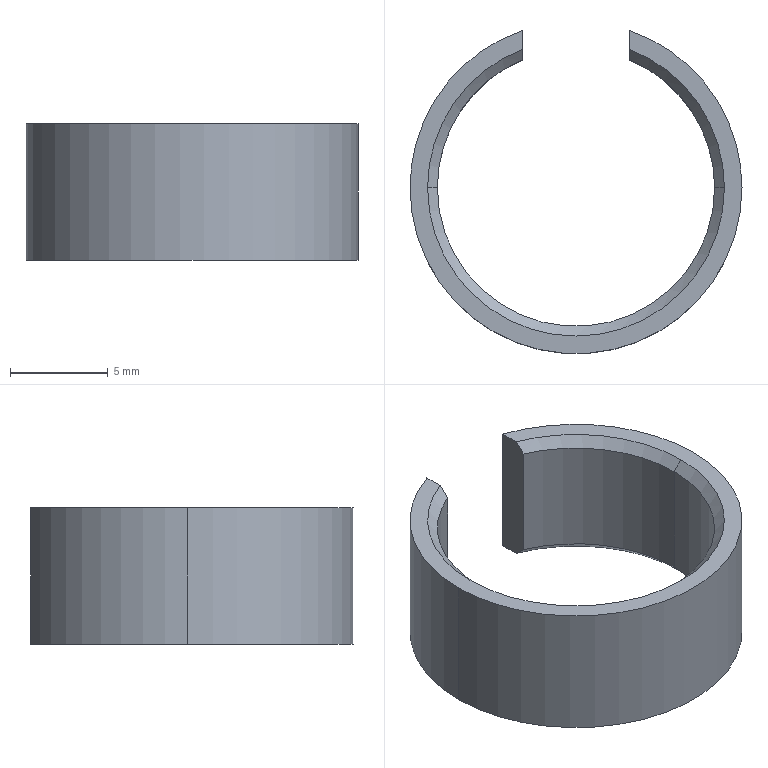Part | SolidWorks | features Chamfer 1, Extrusion 1, ICE 1 | 1 solid | 16 faces | box 17 x 16.543 x 7 mm | volume 415.187 mm3 | cone 6 | cylinder 6 | plane 4 | commonest cylinder face diameters 14.2 x3 17 x3
STEP:
#1=CARTESIAN_POINT('',(-7.1,0.,6.5));
#2=VERTEX_POINT('',#1);
#3=CARTESIAN_POINT('',(7.1,0.,6.5));
#4=VERTEX_POINT('',#3);
#5=CARTESIAN_POINT('',(0.,0.,6.5));
#6=DIRECTION('',(0.,0.,1.));
#7=DIRECTION('',(1.,0.,0.));
#8=AXIS2_PLACEMENT_3D('',#5,#6,#7);
#9=CIRCLE('',#8,7.1);
#10=EDGE_CURVE('',#2,#4,#9,.T.);
#11=ORIENTED_EDGE('',*,*,#10,.F.);
#12=CARTESIAN_POINT('',(-7.6,0.,7.));
#13=VERTEX_POINT('',#12);
#14=CARTESIAN_POINT('',(-7.1,0.,6.5));
#15=DIRECTION('',(-0.7071,0.,0.7071));
#16=VECTOR('',#15,1000.);
#17=LINE('',#14,#16);
#18=EDGE_CURVE('',#2,#13,#17,.T.);
#19=ORIENTED_EDGE('',*,*,#18,.T.);
#20=CARTESIAN_POINT('',(7.6,0.,7.));
#21=VERTEX_POINT('',#20);
#22=CARTESIAN_POINT('',(0.,0.,7.));
#23=DIRECTION('',(0.,0.,-1.));
#24=DIRECTION('',(1.,0.,0.));
#25=AXIS2_PLACEMENT_3D('',#22,#23,#24);
#26=CIRCLE('',#25,7.6);
#27=EDGE_CURVE('',#21,#13,#26,.T.);
#28=ORIENTED_EDGE('',*,*,#27,.F.);
#29=CARTESIAN_POINT('',(7.1,0.,6.5));
#30=DIRECTION('',(0.7071,0.,0.7071));
#31=VECTOR('',#30,1000.);
#32=LINE('',#29,#31);
#33=EDGE_CURVE('',#4,#21,#32,.T.);
#34=ORIENTED_EDGE('',*,*,#33,.F.);
#35=EDGE_LOOP('',(#11,#19,#28,#34));
#36=FACE_OUTER_BOUND('',#35,.T.);
#37=CARTESIAN_POINT('',(0.,0.,6.5));
#38=DIRECTION('',(0.,0.,1.));
#39=DIRECTION('',(1.,0.,0.));
#40=AXIS2_PLACEMENT_3D('',#37,#38,#39);
#41=CONICAL_SURFACE('',#40,7.1,0.7854);
#42=ADVANCED_FACE('',(#36),#41,.F.);
#43=CARTESIAN_POINT('',(2.75,6.546,6.5));
#44=VERTEX_POINT('',#43);
#45=CARTESIAN_POINT('',(0.,0.,6.5));
#46=DIRECTION('',(0.,0.,1.));
#47=DIRECTION('',(1.,0.,0.));
#48=AXIS2_PLACEMENT_3D('',#45,#46,#47);
#49=CIRCLE('',#48,7.1);
#50=EDGE_CURVE('',#4,#44,#49,.T.);
#51=ORIENTED_EDGE('',*,*,#50,.F.);
#52=ORIENTED_EDGE('',*,*,#33,.T.);
#53=CARTESIAN_POINT('',(2.75,7.085,7.));
#54=VERTEX_POINT('',#53);
#55=CARTESIAN_POINT('',(0.,0.,7.));
#56=DIRECTION('',(0.,0.,-1.));
#57=DIRECTION('',(1.,0.,0.));
#58=AXIS2_PLACEMENT_3D('',#55,#56,#57);
#59=CIRCLE('',#58,7.6);
#60=EDGE_CURVE('',#54,#21,#59,.T.);
#61=ORIENTED_EDGE('',*,*,#60,.F.);
#62=CARTESIAN_POINT('',(2.75,6.546,6.5));
#63=CARTESIAN_POINT('',(2.75,6.726,6.666));
#64=CARTESIAN_POINT('',(2.75,6.906,6.833));
#65=CARTESIAN_POINT('',(2.75,7.085,7.));
#66=B_SPLINE_CURVE_WITH_KNOTS('',3,(#62,#63,#64,#65),.UNSPECIFIED.,.F.,.F.,(4,4),(0.,0.0007354),.UNSPECIFIED.);
#67=EDGE_CURVE('',#44,#54,#66,.T.);
#68=ORIENTED_EDGE('',*,*,#67,.F.);
#69=EDGE_LOOP('',(#51,#52,#61,#68));
#70=FACE_OUTER_BOUND('',#69,.T.);
#71=CARTESIAN_POINT('',(0.,0.,6.5));
#72=DIRECTION('',(0.,0.,1.));
#73=DIRECTION('',(1.,0.,0.));
#74=AXIS2_PLACEMENT_3D('',#71,#72,#73);
#75=CONICAL_SURFACE('',#74,7.1,0.7854);
#76=ADVANCED_FACE('',(#70),#75,.F.);
#77=CARTESIAN_POINT('',(7.1,0.,0.5));
#78=VERTEX_POINT('',#77);
#79=CARTESIAN_POINT('',(-7.1,0.,0.5));
#80=VERTEX_POINT('',#79);
#81=CARTESIAN_POINT('',(0.,0.,0.5));
#82=DIRECTION('',(0.,0.,-1.));
#83=DIRECTION('',(1.,0.,0.));
#84=AXIS2_PLACEMENT_3D('',#81,#82,#83);
#85=CIRCLE('',#84,7.1);
#86=EDGE_CURVE('',#78,#80,#85,.T.);
#87=ORIENTED_EDGE('',*,*,#86,.F.);
#88=CARTESIAN_POINT('',(7.6,0.,0.));
#89=VERTEX_POINT('',#88);
#90=CARTESIAN_POINT('',(7.6,0.,0.));
#91=DIRECTION('',(0.7071,0.,-0.7071));
#92=VECTOR('',#91,1000.);
#93=LINE('',#90,#92);
#94=EDGE_CURVE('',#78,#89,#93,.T.);
#95=ORIENTED_EDGE('',*,*,#94,.T.);
#96=CARTESIAN_POINT('',(-7.6,0.,0.));
#97=VERTEX_POINT('',#96);
#98=CARTESIAN_POINT('',(0.,0.,0.));
#99=DIRECTION('',(0.,0.,1.));
#100=DIRECTION('',(1.,0.,0.));
#101=AXIS2_PLACEMENT_3D('',#98,#99,#100);
#102=CIRCLE('',#101,7.6);
#103=EDGE_CURVE('',#97,#89,#102,.T.);
#104=ORIENTED_EDGE('',*,*,#103,.F.);
#105=CARTESIAN_POINT('',(-7.6,0.,0.));
#106=DIRECTION('',(-0.7071,0.,-0.7071));
#107=VECTOR('',#106,1000.);
#108=LINE('',#105,#107);
#109=EDGE_CURVE('',#80,#97,#108,.T.);
#110=ORIENTED_EDGE('',*,*,#109,.F.);
#111=EDGE_LOOP('',(#87,#95,#104,#110));
#112=FACE_OUTER_BOUND('',#111,.T.);
#113=CARTESIAN_POINT('',(0.,0.,0.));
#114=DIRECTION('',(0.,0.,-1.));
#115=DIRECTION('',(-1.,0.,0.));
#116=AXIS2_PLACEMENT_3D('',#113,#114,#115);
#117=CONICAL_SURFACE('',#116,7.6,0.7854);
#118=ADVANCED_FACE('',(#112),#117,.F.);
#119=CARTESIAN_POINT('',(-2.75,6.546,0.5));
#120=VERTEX_POINT('',#119);
#121=CARTESIAN_POINT('',(0.,0.,0.5));
#122=DIRECTION('',(0.,0.,-1.));
#123=DIRECTION('',(1.,0.,0.));
#124=AXIS2_PLACEMENT_3D('',#121,#122,#123);
#125=CIRCLE('',#124,7.1);
#126=EDGE_CURVE('',#80,#120,#125,.T.);
#127=ORIENTED_EDGE('',*,*,#126,.F.);
#128=ORIENTED_EDGE('',*,*,#109,.T.);
#129=CARTESIAN_POINT('',(-2.75,7.085,0.));
#130=VERTEX_POINT('',#129);
#131=CARTESIAN_POINT('',(0.,0.,0.));
#132=DIRECTION('',(0.,0.,1.));
#133=DIRECTION('',(1.,0.,0.));
#134=AXIS2_PLACEMENT_3D('',#131,#132,#133);
#135=CIRCLE('',#134,7.6);
#136=EDGE_CURVE('',#130,#97,#135,.T.);
#137=ORIENTED_EDGE('',*,*,#136,.F.);
#138=CARTESIAN_POINT('',(-2.75,6.546,0.5));
#139=CARTESIAN_POINT('',(-2.75,6.726,0.3338));
#140=CARTESIAN_POINT('',(-2.75,6.906,0.1671));
#141=CARTESIAN_POINT('',(-2.75,7.085,0.));
#142=B_SPLINE_CURVE_WITH_KNOTS('',3,(#138,#139,#140,#141),.UNSPECIFIED.,.F.,.F.,(4,4),(0.,0.0007354),.UNSPECIFIED.);
#143=EDGE_CURVE('',#120,#130,#142,.T.);
#144=ORIENTED_EDGE('',*,*,#143,.F.);
#145=EDGE_LOOP('',(#127,#128,#137,#144));
#146=FACE_OUTER_BOUND('',#145,.T.);
#147=CARTESIAN_POINT('',(0.,0.,0.));
#148=DIRECTION('',(0.,0.,-1.));
#149=DIRECTION('',(-1.,0.,0.));
#150=AXIS2_PLACEMENT_3D('',#147,#148,#149);
#151=CONICAL_SURFACE('',#150,7.6,0.7854);
#152=ADVANCED_FACE('',(#146),#151,.F.);
#153=ORIENTED_EDGE('',*,*,#10,.T.);
#154=CARTESIAN_POINT('',(7.1,0.,7.));
#155=DIRECTION('',(0.,0.,-1.));
#156=VECTOR('',#155,1000.);
#157=LINE('',#154,#156);
#158=EDGE_CURVE('',#4,#78,#157,.T.);
#159=ORIENTED_EDGE('',*,*,#158,.T.);
#160=ORIENTED_EDGE('',*,*,#86,.T.);
#161=CARTESIAN_POINT('',(-7.1,0.,7.));
#162=DIRECTION('',(0.,0.,-1.));
#163=VECTOR('',#162,1000.);
#164=LINE('',#161,#163);
#165=EDGE_CURVE('',#2,#80,#164,.T.);
#166=ORIENTED_EDGE('',*,*,#165,.F.);
#167=EDGE_LOOP('',(#153,#159,#160,#166));
#168=FACE_OUTER_BOUND('',#167,.T.);
#169=CARTESIAN_POINT('',(0.,0.,7.));
#170=DIRECTION('',(0.,0.,-1.));
#171=DIRECTION('',(-1.,0.,0.));
#172=AXIS2_PLACEMENT_3D('',#169,#170,#171);
#173=CYLINDRICAL_SURFACE('',#172,7.1);
#174=ADVANCED_FACE('',(#168),#173,.F.);
#175=CARTESIAN_POINT('',(-2.75,6.546,6.5));
#176=VERTEX_POINT('',#175);
#177=CARTESIAN_POINT('',(0.,0.,6.5));
#178=DIRECTION('',(0.,0.,1.));
#179=DIRECTION('',(1.,0.,0.));
#180=AXIS2_PLACEMENT_3D('',#177,#178,#179);
#181=CIRCLE('',#180,7.1);
#182=EDGE_CURVE('',#176,#2,#181,.T.);
#183=ORIENTED_EDGE('',*,*,#182,.T.);
#184=ORIENTED_EDGE('',*,*,#165,.T.);
#185=ORIENTED_EDGE('',*,*,#126,.T.);
#186=CARTESIAN_POINT('',(-2.75,6.546,7.));
#187=DIRECTION('',(0.,0.,-1.));
#188=VECTOR('',#187,1000.);
#189=LINE('',#186,#188);
#190=EDGE_CURVE('',#176,#120,#189,.T.);
#191=ORIENTED_EDGE('',*,*,#190,.F.);
#192=EDGE_LOOP('',(#183,#184,#185,#191));
#193=FACE_OUTER_BOUND('',#192,.T.);
#194=CARTESIAN_POINT('',(0.,0.,7.));
#195=DIRECTION('',(0.,0.,-1.));
#196=DIRECTION('',(-1.,0.,0.));
#197=AXIS2_PLACEMENT_3D('',#194,#195,#196);
#198=CYLINDRICAL_SURFACE('',#197,7.1);
#199=ADVANCED_FACE('',(#193),#198,.F.);
#200=CARTESIAN_POINT('',(8.5,0.,7.));
#201=VERTEX_POINT('',#200);
#202=CARTESIAN_POINT('',(2.75,8.043,7.));
#203=VERTEX_POINT('',#202);
#204=CARTESIAN_POINT('',(0.,0.,7.));
#205=DIRECTION('',(0.,0.,1.));
#206=DIRECTION('',(1.,0.,0.));
#207=AXIS2_PLACEMENT_3D('',#204,#205,#206);
#208=CIRCLE('',#207,8.5);
#209=EDGE_CURVE('',#201,#203,#208,.T.);
#210=ORIENTED_EDGE('',*,*,#209,.F.);
#211=CARTESIAN_POINT('',(8.5,0.,0.));
#212=VERTEX_POINT('',#211);
#213=CARTESIAN_POINT('',(8.5,0.,7.));
#214=DIRECTION('',(0.,0.,-1.));
#215=VECTOR('',#214,1000.);
#216=LINE('',#213,#215);
#217=EDGE_CURVE('',#201,#212,#216,.T.);
#218=ORIENTED_EDGE('',*,*,#217,.T.);
#219=CARTESIAN_POINT('',(2.75,8.043,0.));
#220=VERTEX_POINT('',#219);
#221=CARTESIAN_POINT('',(0.,0.,0.));
#222=DIRECTION('',(0.,0.,1.));
#223=DIRECTION('',(1.,0.,0.));
#224=AXIS2_PLACEMENT_3D('',#221,#222,#223);
#225=CIRCLE('',#224,8.5);
#226=EDGE_CURVE('',#212,#220,#225,.T.);
#227=ORIENTED_EDGE('',*,*,#226,.T.);
#228=CARTESIAN_POINT('',(2.75,8.043,7.));
#229=DIRECTION('',(0.,0.,1.));
#230=VECTOR('',#229,1000.);
#231=LINE('',#228,#230);
#232=EDGE_CURVE('',#220,#203,#231,.T.);
#233=ORIENTED_EDGE('',*,*,#232,.T.);
#234=EDGE_LOOP('',(#210,#218,#227,#233));
#235=FACE_OUTER_BOUND('',#234,.T.);
#236=CARTESIAN_POINT('',(0.,0.,7.));
#237=DIRECTION('',(0.,0.,-1.));
#238=DIRECTION('',(-1.,0.,0.));
#239=AXIS2_PLACEMENT_3D('',#236,#237,#238);
#240=CYLINDRICAL_SURFACE('',#239,8.5);
#241=ADVANCED_FACE('',(#235),#240,.T.);
#242=ORIENTED_EDGE('',*,*,#217,.F.);
#243=CARTESIAN_POINT('',(-8.5,0.,7.));
#244=VERTEX_POINT('',#243);
#245=CARTESIAN_POINT('',(0.,0.,7.));
#246=DIRECTION('',(0.,0.,1.));
#247=DIRECTION('',(1.,0.,0.));
#248=AXIS2_PLACEMENT_3D('',#245,#246,#247);
#249=CIRCLE('',#248,8.5);
#250=EDGE_CURVE('',#244,#201,#249,.T.);
#251=ORIENTED_EDGE('',*,*,#250,.F.);
#252=CARTESIAN_POINT('',(-8.5,0.,0.));
#253=VERTEX_POINT('',#252);
#254=CARTESIAN_POINT('',(-8.5,0.,7.));
#255=DIRECTION('',(0.,0.,-1.));
#256=VECTOR('',#255,1000.);
#257=LINE('',#254,#256);
#258=EDGE_CURVE('',#244,#253,#257,.T.);
#259=ORIENTED_EDGE('',*,*,#258,.T.);
#260=CARTESIAN_POINT('',(0.,0.,0.));
#261=DIRECTION('',(0.,0.,1.));
#262=DIRECTION('',(1.,0.,0.));
#263=AXIS2_PLACEMENT_3D('',#260,#261,#262);
#264=CIRCLE('',#263,8.5);
#265=EDGE_CURVE('',#253,#212,#264,.T.);
#266=ORIENTED_EDGE('',*,*,#265,.T.);
#267=EDGE_LOOP('',(#242,#251,#259,#266));
#268=FACE_OUTER_BOUND('',#267,.T.);
#269=CARTESIAN_POINT('',(0.,0.,7.));
#270=DIRECTION('',(0.,0.,-1.));
#271=DIRECTION('',(-1.,0.,0.));
#272=AXIS2_PLACEMENT_3D('',#269,#270,#271);
#273=CYLINDRICAL_SURFACE('',#272,8.5);
#274=ADVANCED_FACE('',(#268),#273,.T.);
#275=CARTESIAN_POINT('',(2.75,0.,7.));
#276=DIRECTION('',(0.,1.,0.));
#277=VECTOR('',#276,1000.);
#278=LINE('',#275,#277);
#279=EDGE_CURVE('',#54,#203,#278,.T.);
#280=ORIENTED_EDGE('',*,*,#279,.F.);
#281=ORIENTED_EDGE('',*,*,#60,.T.);
#282=ORIENTED_EDGE('',*,*,#27,.T.);
#283=CARTESIAN_POINT('',(-2.75,7.085,7.));
#284=VERTEX_POINT('',#283);
#285=CARTESIAN_POINT('',(0.,0.,7.));
#286=DIRECTION('',(0.,0.,-1.));
#287=DIRECTION('',(1.,0.,0.));
#288=AXIS2_PLACEMENT_3D('',#285,#286,#287);
#289=CIRCLE('',#288,7.6);
#290=EDGE_CURVE('',#13,#284,#289,.T.);
#291=ORIENTED_EDGE('',*,*,#290,.T.);
#292=CARTESIAN_POINT('',(-2.75,8.043,7.));
#293=VERTEX_POINT('',#292);
#294=CARTESIAN_POINT('',(-2.75,0.,7.));
#295=DIRECTION('',(0.,-1.,0.));
#296=VECTOR('',#295,1000.);
#297=LINE('',#294,#296);
#298=EDGE_CURVE('',#293,#284,#297,.T.);
#299=ORIENTED_EDGE('',*,*,#298,.F.);
#300=CARTESIAN_POINT('',(0.,0.,7.));
#301=DIRECTION('',(0.,0.,1.));
#302=DIRECTION('',(1.,0.,0.));
#303=AXIS2_PLACEMENT_3D('',#300,#301,#302);
#304=CIRCLE('',#303,8.5);
#305=EDGE_CURVE('',#293,#244,#304,.T.);
#306=ORIENTED_EDGE('',*,*,#305,.T.);
#307=ORIENTED_EDGE('',*,*,#250,.T.);
#308=ORIENTED_EDGE('',*,*,#209,.T.);
#309=EDGE_LOOP('',(#280,#281,#282,#291,#299,#306,#307,#308));
#310=FACE_OUTER_BOUND('',#309,.T.);
#311=CARTESIAN_POINT('',(0.,0.,7.));
#312=DIRECTION('',(0.,0.,1.));
#313=DIRECTION('',(1.,0.,0.));
#314=AXIS2_PLACEMENT_3D('',#311,#312,#313);
#315=PLANE('',#314);
#316=ADVANCED_FACE('',(#310),#315,.T.);
#317=CARTESIAN_POINT('',(-2.75,8.043,0.));
#318=VERTEX_POINT('',#317);
#319=CARTESIAN_POINT('',(-2.75,0.,0.));
#320=DIRECTION('',(0.,-1.,0.));
#321=VECTOR('',#320,1000.);
#322=LINE('',#319,#321);
#323=EDGE_CURVE('',#318,#130,#322,.T.);
#324=ORIENTED_EDGE('',*,*,#323,.T.);
#325=ORIENTED_EDGE('',*,*,#136,.T.);
#326=ORIENTED_EDGE('',*,*,#103,.T.);
#327=CARTESIAN_POINT('',(2.75,7.085,0.));
#328=VERTEX_POINT('',#327);
#329=CARTESIAN_POINT('',(0.,0.,0.));
#330=DIRECTION('',(0.,0.,1.));
#331=DIRECTION('',(1.,0.,0.));
#332=AXIS2_PLACEMENT_3D('',#329,#330,#331);
#333=CIRCLE('',#332,7.6);
#334=EDGE_CURVE('',#89,#328,#333,.T.);
#335=ORIENTED_EDGE('',*,*,#334,.T.);
#336=CARTESIAN_POINT('',(2.75,0.,0.));
#337=DIRECTION('',(0.,1.,0.));
#338=VECTOR('',#337,1000.);
#339=LINE('',#336,#338);
#340=EDGE_CURVE('',#328,#220,#339,.T.);
#341=ORIENTED_EDGE('',*,*,#340,.T.);
#342=ORIENTED_EDGE('',*,*,#226,.F.);
#343=ORIENTED_EDGE('',*,*,#265,.F.);
#344=CARTESIAN_POINT('',(0.,0.,0.));
#345=DIRECTION('',(0.,0.,1.));
#346=DIRECTION('',(1.,0.,0.));
#347=AXIS2_PLACEMENT_3D('',#344,#345,#346);
#348=CIRCLE('',#347,8.5);
#349=EDGE_CURVE('',#318,#253,#348,.T.);
#350=ORIENTED_EDGE('',*,*,#349,.F.);
#351=EDGE_LOOP('',(#324,#325,#326,#335,#341,#342,#343,#350));
#352=FACE_OUTER_BOUND('',#351,.T.);
#353=CARTESIAN_POINT('',(0.,0.,0.));
#354=DIRECTION('',(0.,0.,1.));
#355=DIRECTION('',(1.,0.,0.));
#356=AXIS2_PLACEMENT_3D('',#353,#354,#355);
#357=PLANE('',#356);
#358=ADVANCED_FACE('',(#352),#357,.F.);
#359=ORIENTED_EDGE('',*,*,#258,.F.);
#360=ORIENTED_EDGE('',*,*,#305,.F.);
#361=CARTESIAN_POINT('',(-2.75,8.043,7.));
#362=DIRECTION('',(0.,0.,-1.));
#363=VECTOR('',#362,1000.);
#364=LINE('',#361,#363);
#365=EDGE_CURVE('',#293,#318,#364,.T.);
#366=ORIENTED_EDGE('',*,*,#365,.T.);
#367=ORIENTED_EDGE('',*,*,#349,.T.);
#368=EDGE_LOOP('',(#359,#360,#366,#367));
#369=FACE_OUTER_BOUND('',#368,.T.);
#370=CARTESIAN_POINT('',(0.,0.,7.));
#371=DIRECTION('',(0.,0.,-1.));
#372=DIRECTION('',(-1.,0.,0.));
#373=AXIS2_PLACEMENT_3D('',#370,#371,#372);
#374=CYLINDRICAL_SURFACE('',#373,8.5);
#375=ADVANCED_FACE('',(#369),#374,.T.);
#376=ORIENTED_EDGE('',*,*,#158,.F.);
#377=ORIENTED_EDGE('',*,*,#50,.T.);
#378=CARTESIAN_POINT('',(2.75,6.546,0.5));
#379=VERTEX_POINT('',#378);
#380=CARTESIAN_POINT('',(2.75,6.546,7.));
#381=DIRECTION('',(0.,0.,1.));
#382=VECTOR('',#381,1000.);
#383=LINE('',#380,#382);
#384=EDGE_CURVE('',#379,#44,#383,.T.);
#385=ORIENTED_EDGE('',*,*,#384,.F.);
#386=CARTESIAN_POINT('',(0.,0.,0.5));
#387=DIRECTION('',(0.,0.,-1.));
#388=DIRECTION('',(1.,0.,0.));
#389=AXIS2_PLACEMENT_3D('',#386,#387,#388);
#390=CIRCLE('',#389,7.1);
#391=EDGE_CURVE('',#379,#78,#390,.T.);
#392=ORIENTED_EDGE('',*,*,#391,.T.);
#393=EDGE_LOOP('',(#376,#377,#385,#392));
#394=FACE_OUTER_BOUND('',#393,.T.);
#395=CARTESIAN_POINT('',(0.,0.,7.));
#396=DIRECTION('',(0.,0.,-1.));
#397=DIRECTION('',(-1.,0.,0.));
#398=AXIS2_PLACEMENT_3D('',#395,#396,#397);
#399=CYLINDRICAL_SURFACE('',#398,7.1);
#400=ADVANCED_FACE('',(#394),#399,.F.);
#401=ORIENTED_EDGE('',*,*,#340,.F.);
#402=CARTESIAN_POINT('',(2.75,7.085,0.));
#403=CARTESIAN_POINT('',(2.75,6.906,0.1671));
#404=CARTESIAN_POINT('',(2.75,6.726,0.3338));
#405=CARTESIAN_POINT('',(2.75,6.546,0.5));
#406=B_SPLINE_CURVE_WITH_KNOTS('',3,(#402,#403,#404,#405),.UNSPECIFIED.,.F.,.F.,(4,4),(0.,0.0007354),.UNSPECIFIED.);
#407=EDGE_CURVE('',#328,#379,#406,.T.);
#408=ORIENTED_EDGE('',*,*,#407,.T.);
#409=ORIENTED_EDGE('',*,*,#384,.T.);
#410=ORIENTED_EDGE('',*,*,#67,.T.);
#411=ORIENTED_EDGE('',*,*,#279,.T.);
#412=ORIENTED_EDGE('',*,*,#232,.F.);
#413=EDGE_LOOP('',(#401,#408,#409,#410,#411,#412));
#414=FACE_OUTER_BOUND('',#413,.T.);
#415=CARTESIAN_POINT('',(2.75,0.,0.));
#416=DIRECTION('',(1.,0.,0.));
#417=DIRECTION('',(0.,0.,-1.));
#418=AXIS2_PLACEMENT_3D('',#415,#416,#417);
#419=PLANE('',#418);
#420=ADVANCED_FACE('',(#414),#419,.F.);
#421=ORIENTED_EDGE('',*,*,#190,.T.);
#422=ORIENTED_EDGE('',*,*,#143,.T.);
#423=ORIENTED_EDGE('',*,*,#323,.F.);
#424=ORIENTED_EDGE('',*,*,#365,.F.);
#425=ORIENTED_EDGE('',*,*,#298,.T.);
#426=CARTESIAN_POINT('',(-2.75,7.085,7.));
#427=CARTESIAN_POINT('',(-2.75,6.906,6.833));
#428=CARTESIAN_POINT('',(-2.75,6.726,6.666));
#429=CARTESIAN_POINT('',(-2.75,6.546,6.5));
#430=B_SPLINE_CURVE_WITH_KNOTS('',3,(#426,#427,#428,#429),.UNSPECIFIED.,.F.,.F.,(4,4),(0.,0.0007354),.UNSPECIFIED.);
#431=EDGE_CURVE('',#284,#176,#430,.T.);
#432=ORIENTED_EDGE('',*,*,#431,.T.);
#433=EDGE_LOOP('',(#421,#422,#423,#424,#425,#432));
#434=FACE_OUTER_BOUND('',#433,.T.);
#435=CARTESIAN_POINT('',(-2.75,0.,0.));
#436=DIRECTION('',(-1.,0.,0.));
#437=DIRECTION('',(0.,0.,1.));
#438=AXIS2_PLACEMENT_3D('',#435,#436,#437);
#439=PLANE('',#438);
#440=ADVANCED_FACE('',(#434),#439,.F.);
#441=ORIENTED_EDGE('',*,*,#94,.F.);
#442=ORIENTED_EDGE('',*,*,#391,.F.);
#443=ORIENTED_EDGE('',*,*,#407,.F.);
#444=ORIENTED_EDGE('',*,*,#334,.F.);
#445=EDGE_LOOP('',(#441,#442,#443,#444));
#446=FACE_OUTER_BOUND('',#445,.T.);
#447=CARTESIAN_POINT('',(0.,0.,0.));
#448=DIRECTION('',(0.,0.,-1.));
#449=DIRECTION('',(-1.,0.,0.));
#450=AXIS2_PLACEMENT_3D('',#447,#448,#449);
#451=CONICAL_SURFACE('',#450,7.6,0.7854);
#452=ADVANCED_FACE('',(#446),#451,.F.);
#453=ORIENTED_EDGE('',*,*,#18,.F.);
#454=ORIENTED_EDGE('',*,*,#182,.F.);
#455=ORIENTED_EDGE('',*,*,#431,.F.);
#456=ORIENTED_EDGE('',*,*,#290,.F.);
#457=EDGE_LOOP('',(#453,#454,#455,#456));
#458=FACE_OUTER_BOUND('',#457,.T.);
#459=CARTESIAN_POINT('',(0.,0.,6.5));
#460=DIRECTION('',(0.,0.,1.));
#461=DIRECTION('',(1.,0.,0.));
#462=AXIS2_PLACEMENT_3D('',#459,#460,#461);
#463=CONICAL_SURFACE('',#462,7.1,0.7854);
#464=ADVANCED_FACE('',(#458),#463,.F.);
#465=CLOSED_SHELL('',(#42,#76,#118,#152,#174,#199,#241,#274,#316,#358,#375,#400,#420,#440,#452,#464));
#466=MANIFOLD_SOLID_BREP('',#465);
#467=CARTESIAN_POINT('',(0.,0.,0.));
#468=DIRECTION('',(0.,0.,1.));
#469=DIRECTION('',(1.,0.,0.));
#470=AXIS2_PLACEMENT_3D('',#467,#468,#469);
#471=(LENGTH_UNIT()NAMED_UNIT(*)SI_UNIT(.MILLI.,.METRE.));
#472=UNCERTAINTY_MEASURE_WITH_UNIT(LENGTH_MEASURE(0.00001),#471,'','');
#473=(NAMED_UNIT(*)PLANE_ANGLE_UNIT()SI_UNIT($,.RADIAN.));
#474=(NAMED_UNIT(*)SI_UNIT($,.STERADIAN.)SOLID_ANGLE_UNIT());
#475=(GEOMETRIC_REPRESENTATION_CONTEXT(3)GLOBAL_UNCERTAINTY_ASSIGNED_CONTEXT((#472))GLOBAL_UNIT_ASSIGNED_CONTEXT((#471,#473,#474))REPRESENTATION_CONTEXT('',''));
#476=ADVANCED_BREP_SHAPE_REPRESENTATION('',(#466,#470),#475);